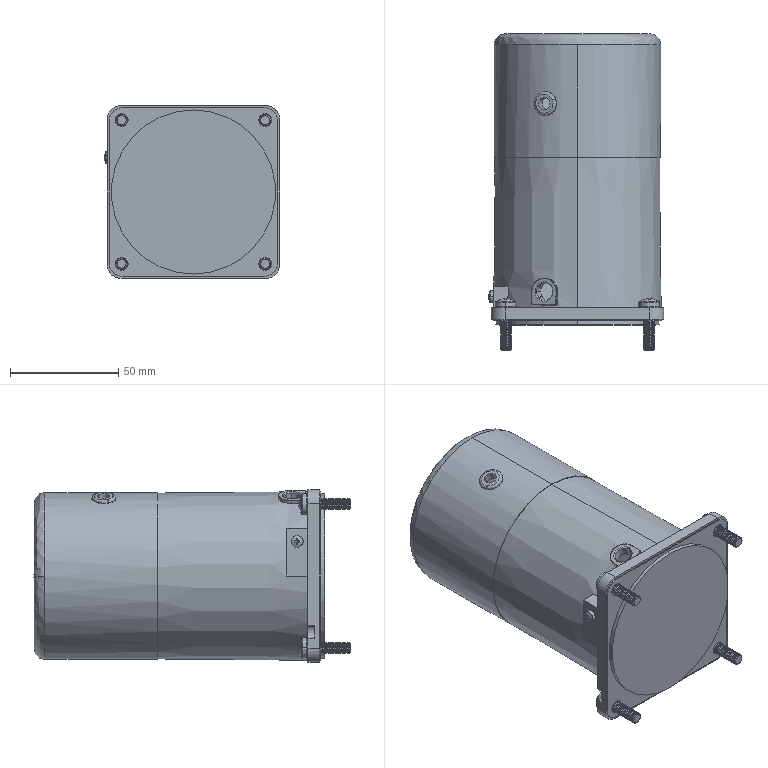Part | SolidWorks | 10 solids | 1306 faces | box 81.301 x 146.321 x 79.972 mm | volume 169247 mm3 | cone 670 | cylinder 373 | plane 186 | spline 77 | commonest cylinder face diameters 5 x192 4 x88 3 x32 8 x8 9.5 x8 10.4 x7